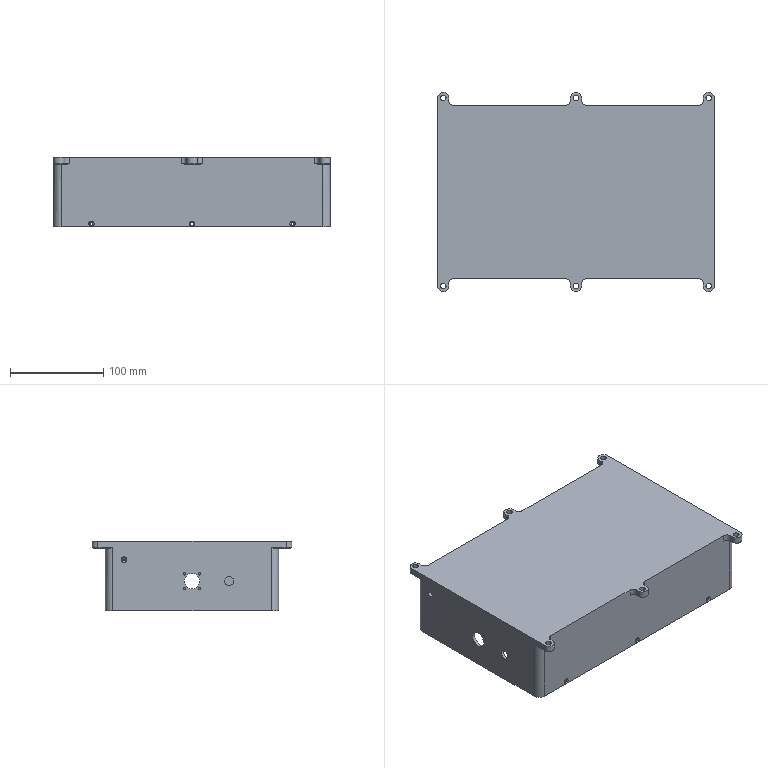Part | 1 solid | 201 faces | box 297 x 214 x 75 mm | volume 379685 mm3 | cylinder 100 | plane 51 | cone 50 | commonest cylinder face diameters 6 x24 10 x17 2.05 x12 3.4 x12 12 x11 16 x11